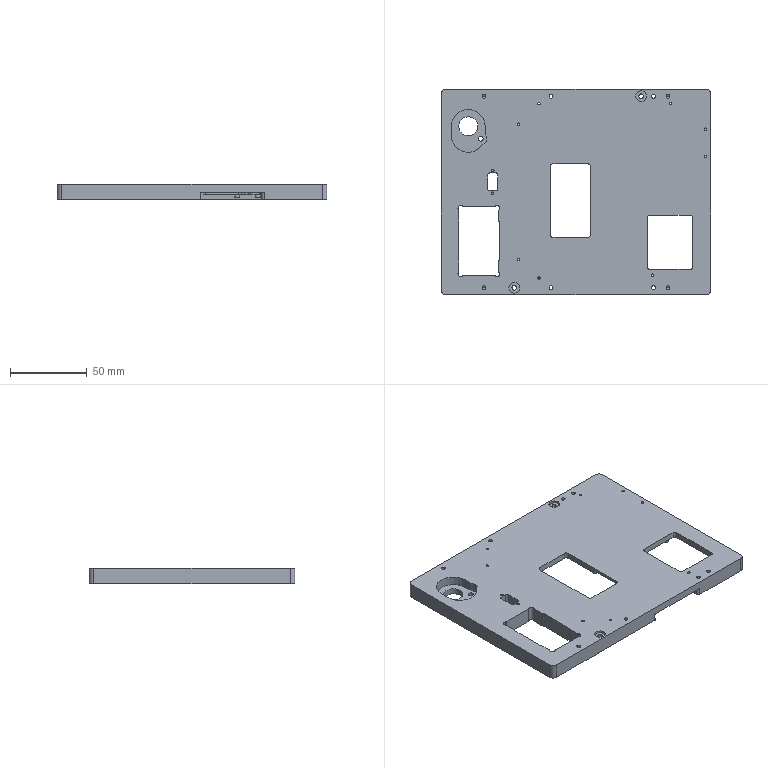NC program | NX | posted with a generic post | part box 176 x 134 x 10 mm
Lines 124 to 1003 of 8914:
(ADAPTIVE_MILLING_COPY , TOOL : D10)
N216 T04 M6
N218 G54
N220 G17 G0 G90 X-60.526 Y-37.7 S9500 M3
N222 G43 Z30. H4
N224 Z1.
N226 G94 G3 X-60.526 Y-37.7 Z0.605 I-2.901 J-3.44 F1000.
N228 X-60.526 Y-37.7 Z0.21 I-2.901 J-3.44
N230 X-60.526 Y-37.7 Z-0.184 I-2.901 J-3.44
N232 X-60.526 Y-37.7 Z-0.579 I-2.901 J-3.44
N234 X-60.526 Y-37.7 Z-0.974 I-2.901 J-3.44
N236 X-60.526 Y-37.7 Z-1.369 I-2.901 J-3.44
N238 X-60.526 Y-37.7 Z-1.764 I-2.901 J-3.44
N240 X-60.526 Y-37.7 Z-2.158 I-2.901 J-3.44
N242 X-60.526 Y-37.7 Z-2.553 I-2.901 J-3.44
N244 X-60.526 Y-37.7 Z-2.948 I-2.901 J-3.44
N246 X-60.526 Y-37.7 Z-3.343 I-2.901 J-3.44
N248 X-60.526 Y-37.7 Z-3.738 I-2.901 J-3.44
N250 X-60.526 Y-37.7 Z-4.133 I-2.901 J-3.44
N252 X-60.526 Y-37.7 Z-4.527 I-2.901 J-3.44
N254 X-60.526 Y-37.7 Z-4.922 I-2.901 J-3.44
N256 X-60.526 Y-37.7 Z-5.317 I-2.901 J-3.44
N258 X-60.526 Y-37.7 Z-5.712 I-2.901 J-3.44
N260 X-60.526 Y-37.7 Z-6.107 I-2.901 J-3.44
N262 X-60.526 Y-37.7 Z-6.501 I-2.901 J-3.44
N264 X-60.526 Y-37.7 Z-6.896 I-2.901 J-3.44
N266 X-60.526 Y-37.7 Z-7.291 I-2.901 J-3.44
N268 X-60.526 Y-37.7 Z-7.686 I-2.901 J-3.44
N270 X-60.526 Y-37.7 Z-8.081 I-2.901 J-3.44
N272 X-60.526 Y-37.7 Z-8.475 I-2.901 J-3.44
N274 X-60.526 Y-37.7 Z-8.87 I-2.901 J-3.44
N276 X-60.526 Y-37.7 Z-9.265 I-2.901 J-3.44
N278 X-60.526 Y-37.7 Z-9.66 I-2.901 J-3.44
N280 X-58.927 Y-41.139 Z-10. R-4.5
N282 X-59.748 Y-43.745 R-4.501 F3500.
N284 X-64.42 Y-36.268 R4.672
N286 X-59.622 Y-44.378 R-4.977
N288 X-65.395 Y-36.044 R5.193
N290 X-59.743 Y-45.214 R-5.474
N292 X-65.843 Y-35.666 R5.72
N294 X-59.62 Y-45.805 R-5.999
N296 X-66.374 Y-35.324 R6.26
N298 X-59.759 Y-46.576 R-6.537
N300 X-66.328 Y-34.682 R6.811
N302 X-59.559 Y-47.121 R-7.099
N304 X-66.7 Y-34.219 R7.384
N306 X-59.276 Y-47.637 R-7.681
N308 X-66.061 Y-33.324 R7.97
N310 X-59.599 Y-48.511 R-8.275
N312 X-57.595 Y-47.115 R8.881
N314 X-55.077 Y-42.632 R7.851
N316 X-55.163 Y-39.012 R27.589
N318 X-63.36 Y-32.265 R8.364
N320 X-71.76 Y-38.033 R8.779
N322 G1 X-71.777 Y-38.154
N324 Y-42.632
N326 G3 X-71.201 Y-45.028 R69.844
N328 X-66.556 Y-49.467 R7.794
N330 X-60.923 Y-49.446 R73.026
N332 X-55.582 Y-45.669 R7.836
N334 X-55.5 Y-45.004 R2.511
N336 G2 X-55.347 Y-43.718 R33.779
N338 G1 X-55.119 Y-42.926
N340 X-55.077 Y-42.632
N342 Y-39.882
N344 G3 X-55.201 Y-37.393 R10.744
N346 X-59.653 Y-32.442 R7.859
N348 X-71.691 Y-36.326 R9.413
N350 G1 X-71.733 Y-36.444
N352 X-71.762 Y-36.566
N354 X-71.777 Y-36.674
N356 Y-38.174
N358 G3 X-71.227 Y-39.126 R1.112
N360 X-70.493 Y-39.275 Z-9.962 R1.332
N362 G1 X-69.254 Y-39.282 Z-9.9
N364 X-57.588 Y-39.349
N366 X-56.035 Y-39.348 Z-9.978
N368 X-55.819 Y-39.293 Z-9.989
N370 X-55.616 Y-39.203 Z-10.
N372 G3 X-55.077 Y-38.257 R1.112
N374 X-55.483 Y-35.569 R5.641
N376 X-61.149 Y-31.221 R8.413
N378 X-71.65 Y-35.064 R9.921
N380 G1 X-71.701 Y-35.178
N382 X-71.74 Y-35.297
N384 X-71.767 Y-35.419
N386 X-71.777 Y-35.493
N388 Y-36.743
N390 G3 X-71.229 Y-37.695 R1.112
N392 X-70.513 Y-37.848 Z-9.963 R1.365
N394 G1 X-69.256 Y-37.882 Z-9.9
N396 X-57.588 Y-38.195
N398 X-56.82 Y-38.218 Z-9.938
N400 X-56.052 Y-38.225 Z-9.977
N402 X-55.827 Y-38.171 Z-9.988
N404 X-55.616 Y-38.078 Z-10.
N406 G3 X-55.077 Y-37.132 R1.112
N408 X-56.62 Y-33.066 R4.979
N410 X-65.601 Y-30.438 R9.835
N412 X-71.544 Y-33.867 R10.035
N414 X-71.777 Y-34.459 R1.804
N416 G1 Y-35.584
N418 G3 X-71.23 Y-36.535 R1.112
N420 X-70.532 Y-36.692 Z-9.964 R1.388
N422 G1 X-69.258 Y-36.751 Z-9.9
N424 X-57.587 Y-37.293
N426 X-56.828 Y-37.332 Z-9.938
N428 X-56.068 Y-37.352 Z-9.976
N430 X-55.835 Y-37.299 Z-9.988
N432 X-55.616 Y-37.204 Z-10.
N434 G3 X-55.077 Y-36.257 R1.112
N436 X-56.507 Y-32.407 R4.688
N438 X-64.492 Y-29.582 R9.928
N440 X-71.39 Y-32.726 R10.586
N442 X-71.777 Y-33.511 R1.491
N444 G1 Y-34.511
N446 G3 X-71.231 Y-35.462 R1.112
N448 X-70.537 Y-35.62 Z-9.964 R1.393
N450 G1 X-69.26 Y-35.686 Z-9.9
N452 X-57.587 Y-36.286
N454 X-56.83 Y-36.329 Z-9.938
N456 X-56.073 Y-36.352 Z-9.976
N458 X-55.838 Y-36.3 Z-9.988
N460 X-55.617 Y-36.204 Z-10.
N462 G3 X-55.077 Y-35.257 R1.112
N464 X-56.412 Y-31.751 R4.409
N466 X-63.51 Y-28.846 R9.893
N468 X-71.115 Y-31.539 R11.237
N470 X-71.777 Y-32.609 R1.829
N472 G1 Y-33.609
N474 G3 X-71.232 Y-34.559 R1.112
N476 X-70.547 Y-34.719 Z-9.964 R1.406
N478 G1 X-69.261 Y-34.798 Z-9.9
N480 X-57.587 Y-35.522
N482 X-56.835 Y-35.573 Z-9.938
N484 X-56.081 Y-35.603 Z-9.975
N486 X-55.842 Y-35.551 Z-9.988
N488 X-55.617 Y-35.454 Z-10.
N490 G3 X-55.077 Y-34.507 R1.112
N492 X-56.413 Y-31.006 R4.337
N494 X-63.408 Y-28.14 R10.025
N496 X-70.99 Y-30.562 R11.468
N498 X-71.777 Y-31.742 R1.951
N500 G1 Y-32.617
N502 G3 X-71.231 Y-33.567 R1.112
N504 X-70.482 Y-33.736 Z-9.961 R1.631
N506 G1 X-69.263 Y-33.832 Z-9.9
N508 X-57.587 Y-34.75
N510 X-56.842 Y-34.813 Z-9.937
N512 X-56.095 Y-34.854 Z-9.975
N514 X-55.849 Y-34.803 Z-9.987
N516 X-55.618 Y-34.705 Z-10.
N518 G3 X-55.077 Y-33.757 R1.112
N520 X-56.421 Y-30.263 R4.261
N522 X-63.059 Y-27.444 R10.076
N524 X-70.846 Y-29.609 R11.73
N526 X-71.755 Y-30.768 R2.336
N528 G1 X-71.777 Y-30.901
N530 Y-31.776
N532 G3 X-71.232 Y-32.726 R1.112
N534 X-70.488 Y-32.896 Z-9.961 R1.643
N536 G1 X-69.264 Y-33. Z-9.9
N538 X-57.586 Y-33.991
N540 X-56.844 Y-34.059 Z-9.937
N542 X-56.101 Y-34.105 Z-9.975
N544 X-55.852 Y-34.054 Z-9.987
N546 X-55.619 Y-33.955 Z-10.
N548 G3 X-55.077 Y-33.007 R1.112
N550 X-56.435 Y-29.521 R4.229
N552 X-62.964 Y-26.734 R10.188
N554 X-70.695 Y-28.674 R11.94
N556 X-71.742 Y-29.881 R2.605
N558 X-71.777 Y-30.943 R12.814
N560 X-71.233 Y-31.892 R1.112
N562 X-70.493 Y-32.064 Z-9.962 R1.655
N564 G1 X-69.265 Y-32.175 Z-9.9
N566 X-57.586 Y-33.234
N568 X-56.847 Y-33.306 Z-9.937
N570 X-56.105 Y-33.355 Z-9.974
N572 X-55.854 Y-33.305 Z-9.987
N574 X-55.619 Y-33.205 Z-10.
N576 G3 X-55.077 Y-32.257 R1.112
N578 X-56.367 Y-28.87 R4.151
N580 X-62.62 Y-26.045 R10.135
N582 X-70.534 Y-27.751 R12.233
N584 X-71.724 Y-28.998 R2.96
N586 X-71.777 Y-30.122 R5.056
N588 X-71.233 Y-31.071 R1.112
N590 X-70.498 Y-31.244 Z-9.962 R1.665
N592 G1 X-69.267 Y-31.362 Z-9.9
N594 X-57.586 Y-32.478
N596 X-56.849 Y-32.553 Z-9.937
N598 X-56.11 Y-32.605 Z-9.974
N600 X-55.857 Y-32.556 Z-9.987
N602 X-55.619 Y-32.455 Z-10.
N604 G3 X-55.077 Y-31.507 R1.112
N606 X-56.389 Y-28.13 R4.127
N608 X-62.652 Y-25.318 R10.251
N610 X-70.47 Y-26.912 R12.253
N612 X-71.699 Y-28.127 R3.313
N614 X-71.777 Y-29.323 R3.839
N616 X-71.234 Y-30.271 R1.112
N618 X-70.501 Y-30.446 Z-9.962 R1.67
N620 G1 X-69.268 Y-30.568 Z-9.9
N622 X-57.586 Y-31.723
N624 X-56.85 Y-31.801 Z-9.937
N626 X-56.112 Y-31.855 Z-9.974
N628 X-55.858 Y-31.806 Z-9.987
N630 X-55.62 Y-31.706 Z-10.
N632 G3 X-55.077 Y-30.757 R1.112
N634 X-56.328 Y-27.482 R4.053
N636 X-62.312 Y-24.634 R10.179
N638 X-70.296 Y-26.011 R12.507
N640 X-71.716 Y-27.375 R3.296
N642 X-71.777 Y-28.523 R4.403
N644 X-71.235 Y-29.471 R1.112
N646 X-70.504 Y-29.646 Z-9.962 R1.677
N648 G1 X-69.27 Y-29.772 Z-9.9
N650 X-57.586 Y-30.969
N652 X-56.852 Y-31.049 Z-9.937
N654 X-56.115 Y-31.105 Z-9.974
N656 X-55.86 Y-31.057 Z-9.987
N658 X-55.62 Y-30.956 Z-10.
N660 G3 X-55.077 Y-30.007 R1.112
N662 X-56.351 Y-26.742 R4.055
N664 X-62.342 Y-23.901 R10.294
N666 X-70.329 Y-25.253 R12.429
N668 X-71.687 Y-26.512 R3.536
N670 X-71.777 Y-27.747 R3.599
N672 X-71.236 Y-28.695 R1.112
N674 X-70.506 Y-28.871 Z-9.962 R1.678
N676 G1 X-69.271 Y-29. Z-9.9
N678 X-57.586 Y-30.216
N680 X-56.853 Y-30.298 Z-9.937
N682 X-56.117 Y-30.356 Z-9.974
N684 X-55.861 Y-30.307 Z-9.987
N686 X-55.62 Y-30.206 Z-10.
N688 G3 X-55.077 Y-29.257 R1.112
N690 X-56.373 Y-26.001 R4.046
N692 X-62.493 Y-23.147 R10.496
N694 X-70.252 Y-24.428 R12.459
N696 X-71.701 Y-25.765 R3.436
N698 X-71.777 Y-26.956 R3.873
N700 X-71.235 Y-27.904 R1.112
N702 X-70.516 Y-28.082 Z-9.963 R1.709
N704 G1 X-69.273 Y-28.226 Z-9.9
N706 X-57.586 Y-29.577
N708 X-56.857 Y-29.667 Z-9.937
N710 X-56.126 Y-29.731 Z-9.973
N712 X-55.866 Y-29.684 Z-9.987
N714 X-55.621 Y-29.582 Z-10.
N716 G3 X-55.077 Y-28.632 R1.112
N718 X-56.397 Y-25.26 R4.101
N720 X-62.521 Y-22.409 R10.57
N722 X-70.282 Y-23.67 R12.37
N724 X-71.714 Y-25.02 R3.246
N726 X-71.777 Y-26.172 R4.315
N728 X-71.236 Y-27.119 R1.112
N730 X-70.519 Y-27.298 Z-9.963 R1.713
N732 G1 X-69.274 Y-27.445 Z-9.9
N734 X-57.586 Y-28.824
N736 X-56.858 Y-28.915 Z-9.937
N738 X-56.128 Y-28.981 Z-9.973
N740 X-55.867 Y-28.934 Z-9.987
N742 X-55.622 Y-28.832 Z-10.
N744 G3 X-55.077 Y-27.882 R1.112
N746 X-56.335 Y-24.61 R4.061
N748 X-62.301 Y-21.707 R10.495
N750 X-70.201 Y-22.851 R12.49
N752 X-71.681 Y-24.159 R3.707
N754 X-71.777 Y-25.397 R3.425
N756 X-71.237 Y-26.344 R1.112
N758 X-70.52 Y-26.524 Z-9.963 R1.714
N760 G1 X-69.276 Y-26.673 Z-9.9
N762 X-57.586 Y-28.071
N764 X-56.859 Y-28.164 Z-9.937
N766 X-56.13 Y-28.231 Z-9.973
N768 X-55.868 Y-28.184 Z-9.987
N770 X-55.622 Y-28.082 Z-10.
N772 G3 X-55.077 Y-27.132 R1.112
N774 X-56.271 Y-23.96 R3.998
N776 X-62.078 Y-21.009 R10.386
N778 X-70.117 Y-22.036 R12.588
N780 X-71.693 Y-23.414 R3.623
N782 X-71.777 Y-24.63 R3.721
N784 X-71.238 Y-25.576 R1.112
N786 X-70.522 Y-25.756 Z-9.963 R1.714
N788 G1 X-69.277 Y-25.907 Z-9.9
N790 X-57.586 Y-27.32
N792 X-56.86 Y-27.413 Z-9.937
N794 X-56.131 Y-27.481 Z-9.973
N796 X-55.868 Y-27.434 Z-9.987
N798 X-55.622 Y-27.332 Z-10.
N800 G3 X-55.077 Y-26.382 R1.112
N802 X-56.377 Y-23.124 R4.098
N804 X-62.471 Y-20.202 R10.732
N806 X-70.139 Y-21.285 R12.45
N808 X-71.703 Y-22.674 R3.454
N810 X-71.777 Y-23.859 R3.92
N812 X-71.238 Y-24.805 R1.112
N814 X-70.531 Y-24.987 Z-9.963 R1.744
N816 G1 X-69.278 Y-25.151 Z-9.9
N818 X-57.586 Y-26.682
N820 X-56.864 Y-26.783 Z-9.936
N822 X-56.139 Y-26.857 Z-9.973
N824 X-55.873 Y-26.811 Z-9.986
N826 X-55.623 Y-26.708 Z-10.
N828 G3 X-55.077 Y-25.757 R1.112
N830 X-56.396 Y-22.382 R4.152
N832 X-62.367 Y-19.48 R10.737
N834 X-70.16 Y-20.532 R12.405
N836 X-71.663 Y-21.816 R3.969
N838 X-71.777 Y-23.092 R3.128
N840 X-71.239 Y-24.037 R1.112
N842 X-70.532 Y-24.22 Z-9.963 R1.744
N844 G1 X-69.28 Y-24.386 Z-9.9
N846 X-57.586 Y-25.931
N848 X-56.865 Y-26.032 Z-9.936
N850 X-56.14 Y-26.107 Z-9.973
N852 X-55.874 Y-26.061 Z-9.986
N854 X-55.623 Y-25.958 Z-10.
N856 G3 X-55.077 Y-25.007 R1.112
N858 X-56.328 Y-21.729 R4.106
N860 X-62.264 Y-18.757 R10.652
N862 X-70.069 Y-19.721 R12.454
N864 X-71.673 Y-21.072 R3.897
N866 X-71.777 Y-22.326 R3.279
N868 X-71.24 Y-23.271 R1.112
N870 X-70.533 Y-23.455 Z-9.963 R1.744
N872 G1 X-69.281 Y-23.622 Z-9.9
N874 X-57.586 Y-25.179
N876 X-56.865 Y-25.281 Z-9.936
N878 X-56.141 Y-25.357 Z-9.973
N880 G3 X-55.624 Y-25.208 Z-10. R1.225
N882 X-55.077 Y-24.257 R1.112
N884 X-56.343 Y-20.986 R4.1
N886 X-62.279 Y-18.013 R10.701
N888 X-70.084 Y-18.97 R12.44
N890 X-71.431 Y-20.051 R3.216
N892 X-71.777 Y-21.472 R5.253
N894 X-71.24 Y-22.417 R1.112
N896 X-70.54 Y-22.602 Z-9.964 R1.765
N898 G1 X-69.283 Y-22.778 Z-9.9
N900 X-57.585 Y-24.42
N902 X-56.184 Y-24.607 Z-9.971
N904 G3 X-55.625 Y-24.458 Z-10. R1.162
N906 X-55.077 Y-23.507 R1.112
N908 X-56.358 Y-20.241 R4.117
N910 X-62.419 Y-17.245 R10.843
N912 X-70.101 Y-18.22 R12.39
N914 X-71.322 Y-19.253 R2.703
N916 X-71.508 Y-20.261 R8.917
N918 X-71.198 Y-21.372 R1.112
N920 X-70.436 Y-21.683 Z-9.958 R1.299
N922 G1 X-69.29 Y-21.869 Z-9.9
N924 X-57.591 Y-23.767
N926 X-56.205 Y-23.982 Z-9.97
N928 G3 X-55.633 Y-23.838 Z-10. R1.16
N930 X-55.077 Y-22.882 R1.112
N932 X-56.373 Y-19.496 R4.179
N934 X-62.557 Y-16.479 R10.927
N936 X-70.002 Y-17.421 R12.259
N938 X-71.285 Y-18.561 R2.598
N940 X-71.413 Y-19.597 R8.909
N942 X-71.052 Y-20.519 R1.116
N944 X-70.309 Y-20.817 Z-9.959 R1.32
N946 G1 X-69.141 Y-21.018 Z-9.9
N948 X-57.586 Y-23.006
N950 X-56.213 Y-23.232 Z-9.97
N952 G3 X-55.631 Y-23.087 Z-10. R1.157
N954 X-55.077 Y-22.132 R1.112
N956 X-56.455 Y-18.689 R4.303
N958 X-62.539 Y-15.739 R10.921
N960 X-69.87 Y-16.612 R12.19
N962 X-71.266 Y-17.817 R3.034
N964 X-71.352 Y-18.915 R3.24
N966 X-70.907 Y-19.798 R1.116
N968 X-70.214 Y-20.031 Z-9.963 R1.366
N970 G1 X-68.967 Y-20.206 Z-9.9
N972 X-57.585 Y-21.808
N974 X-56.941 Y-21.904 Z-9.933
N976 X-56.294 Y-21.976 Z-9.965
N978 G3 X-55.647 Y-21.751 Z-10. R1.145
N980 X-55.257 Y-20.572 R1.108
N982 X-55.701 Y-19.097 R8.228
N984 X-59.336 Y-15.975 R7.604
N986 X-69.431 Y-15.662 R12.888
N988 X-71.212 Y-16.988 R4.158
N990 X-71.352 Y-18.2 R2.531
N992 X-70.854 Y-19.121 R1.115
N994 X-70.116 Y-19.328 Z-9.961 R1.636
N996 G1 X-68.902 Y-19.489 Z-9.9
N998 X-57.753 Y-20.966
N1000 X-57.115 Y-21.056 Z-9.932
N1002 X-56.474 Y-21.122 Z-9.965
N1004 G3 X-55.818 Y-20.88 Z-10. R1.143
N1006 X-55.411 Y-19.919 R1.115
N1008 X-56.909 Y-16.868 R4.192
N1010 X-61.522 Y-14.489 R10.178
N1012 X-67.52 Y-14.527 R124.061
N1014 X-71.098 Y-16.125 R5.682
N1016 X-71.352 Y-16.745 R1.597
N1018 G1 Y-17.495
N1020 G3 X-70.818 Y-18.439 R1.112
N1022 X-70.114 Y-18.625 Z-9.963 R1.753
N1024 G1 X-68.86 Y-18.799 Z-9.9
N1026 X-57.883 Y-20.327
N1028 X-57.219 Y-20.423 Z-9.934
N1030 X-56.552 Y-20.5 Z-9.967
N1032 G3 X-55.936 Y-20.302 Z-10. R1.149
N1034 X-55.47 Y-19.297 R1.112
N1036 X-56.874 Y-16.21 R4.084
N1038 X-59.464 Y-14.506 R7.234
N1040 G1 X-59.583 Y-14.489
N1042 X-61.583
N1044 G3 X-62.179 Y-16.514 R1.101
N1046 G1 X-57.198 Y-19.725
N1048 G3 X-55.502 Y-18.8 R1.102
N1050 X-56.733 Y-15.648 R3.909
N1052 X-58.212 Y-14.524 R4.082
N1054 X-59.646 Y-14.489 R15.119
N1056 X-60.338 Y-16.445 R1.101
N1058 G1 X-57.294 Y-18.906
N1060 G3 X-55.502 Y-18.05 R1.101
N1062 X-57.172 Y-14.614 R3.838
N1064 X-58.47 Y-14.489 R3.013
N1066 X-59.241 Y-16.374 R1.101
N1068 G1 X-57.373 Y-18.21
N1070 G3 X-55.502 Y-17.425 R1.101
N1072 X-56.467 Y-14.704 R3.258
N1074 X-57.671 Y-14.489 R1.91
N1076 X-58.455 Y-16.361 R1.101
N1078 G1 X-57.864 Y-16.97
N1080 X-57.255 Y-17.56
N1082 G3 X-55.502 Y-16.675 R1.101
N1084 X-55.909 Y-14.89 R2.655
N1086 X-57.049 Y-14.489 R1.297
N1088 X-57.839 Y-16.355 R1.101
N1090 G1 X-57.261 Y-16.931
N1092 G3 X-55.502 Y-16.05 R1.101
N1094 X-55.813 Y-14.801 R1.603
N1096 X-56.69 Y-14.489 R1.201
N1098 G1 X-67.022
N1100 G3 X-69.388 Y-14.596 R10.723
N1102 X-71.241 Y-15.769 R2.864
N1104 X-71.352 Y-16.788 R2.415
N1106 X-69.594 Y-17.669 R1.101
N1108 G1 X-67.989 Y-16.471
N1110 G3 X-68.647 Y-14.489 R1.101
N1112 X-70.491 Y-14.703 R4.226
N1114 X-71.352 Y-16.251 R1.39
N1116 X-69.513 Y-17.066 R1.101
N1118 G1 X-69.081 Y-16.679
N1120 X-68.662 Y-16.276
N1122 G3 X-69.522 Y-14.489 R1.101
N1124 X-70.86 Y-14.685 R2.425
N1126 X-71.352 Y-15.802 R1.202
N1128 X-68.865 Y-15.797 R1.244
N1130 X-70.147 Y-14.489 R1.287
N1132 X-71.332 Y-15.401 R1.079
N1134 X-70.654 Y-16.481 R1.007
N1136 G1 X-70.323 Y-16.533 Z-9.983
N1138 X-69.987 Z-9.966
N1140 G2 X-69.281 Y-16.637 Z-9.93 R1.505
N1142 X-68.849 Y-17.048 Z-9.9 R1.047
N1144 G1 X-68.758 Y-17.286
N1146 X-68.723 Y-17.537
N1148 X-68.815 Y-41.972
N1150 G2 X-69.16 Y-42.724 R1.025
N1152 X-69.997 Y-42.968 Z-9.945 R1.137
N1154 G1 X-70.343 Y-42.962 Z-9.962
N1156 X-70.687 Y-42.999 Z-9.979
N1158 X-70.879 Y-43.068 Z-9.99
N1160 X-71.055 Y-43.172 Z-10.
N1162 G3 X-71.443 Y-44.059 R1.014
N1164 X-70.943 Y-46.487 R6.28
N1166 X-68. Y-49.449 R6.448
N1168 X-66.413 Y-49.489 R10.999
N1170 X-65.691 Y-47.559 R1.101
N1172 G1 X-69.531 Y-44.223
N1174 G3 X-71.352 Y-45.054 R1.101
N1176 X-69.896 Y-48.766 R4.582
N1178 X-68.749 Y-49.489 R2.012
N1180 G1 X-67.749
N1182 G3 X-66.958 Y-47.624 R1.101
N1184 G1 X-69.462 Y-45.038
N1186 G3 X-71.352 Y-45.804 R1.101
N1188 X-70.015 Y-49.279 R4.089
N1190 X-69.439 Y-49.489 R1.92
N1192 G1 X-68.689
N1194 G3 X-67.877 Y-47.647 R1.101
N1196 G1 X-69.44 Y-45.937
N1198 G3 X-71.352 Y-46.679 R1.101
N1200 X-70.752 Y-49.04 R3.386
N1202 X-69.942 Y-49.489 R1.225
N1204 G1 X-69.317
N1206 G3 X-68.529 Y-47.622 R1.101
N1208 G1 X-69.053 Y-47.076
N1210 X-69.594 Y-46.547
N1212 G3 X-71.352 Y-47.429 R1.101
N1214 X-71.084 Y-49.002 R2.696
N1216 X-69.873 Y-49.489 R1.267
N1218 X-69.338 Y-47.428 R1.101
N1220 G1 X-69.877 Y-47.144
N1222 G3 X-71.352 Y-48.179 R1.102
N1224 X-70.165 Y-49.489 R1.125
N1226 G1 X-61.42
N1228 G3 X-58.945 Y-49.267 R7.284
N1230 X-55.611 Y-46.75 R6.722
N1232 G1 X-55.564 Y-46.634
N1234 X-55.529 Y-46.514
N1236 X-55.506 Y-46.391
N1238 X-55.502 Y-46.362
N1240 Y-45.237
N1242 G3 X-57.33 Y-44.412 R1.101
N1244 G1 X-60.899 Y-47.565
N1246 G3 X-60.17 Y-49.489 R1.101
N1248 X-57.6 Y-49.123 R5.559
N1250 X-55.641 Y-47.618 R4.794
N1252 X-55.502 Y-46.285 R2.893
N1254 X-57.32 Y-45.452 R1.101
N1256 G1 X-59.763 Y-47.556
N1258 G3 X-59.045 Y-49.489 R1.101
N1260 X-55.998 Y-48.639 R4.266
N1262 X-55.502 Y-47.782 R1.3
N1264 G1 Y-47.157
N1266 G3 X-57.282 Y-46.292 R1.101
N1268 G1 X-58.85 Y-47.525
N1270 G3 X-58.17 Y-49.489 R1.101
N1272 X-56.221 Y-49.19 R3.765
N1274 X-55.502 Y-47.711 R1.383
N1276 X-57.372 Y-46.925 R1.101
N1278 G1 X-57.782 Y-47.322
N1280 X-58.179 Y-47.734
N1282 G3 X-57.295 Y-49.489 R1.101
N1284 X-55.965 Y-49.266 R2.247
N1286 X-55.502 Y-48.177 R1.204
N1288 X-57.898 Y-47.88 R1.217
N1290 X-56.67 Y-49.489 R1.276
N1292 X-55.506 Y-48.454 R1.078
N1294 X-57.238 Y-47.454 R1.42
N1296 G1 Z-7.
N1298 G0 Z30.
N1300 X-99.709 Y-0.062
N1302 Z-9.
N1304 G1 Z-10. F1000.
N1306 X-98.929 Y-0.342 F3500.
N1308 X-98.14 Y-0.598
N1310 G3 X-97.062 Y-0.062 R1.017
N1312 X-96.301 Y3.001 R8.28
N1314 X-96.019 Y12.869 R111.643
N1316 G1 X-96.014 Y15.119
N1318 X-96.011 Y18.994
N1320 X-96.01 Y32.619
N1322 Y67.869
N1324 Y67.994
N1326 X-96.008 Y68.119
N1328 G2 X-93.514 Y72.4 R5.714
N1330 X-88.075 Y74.465 R12.318
N1332 X-79.847 Y74.954 R58.201
N1334 G1 X-78.722 Y74.965
N1336 X-77.347 Y74.974
N1338 X-75.722 Y74.98
N1340 X-73.347 Y74.985
N1342 X-69.222 Y74.987
N1344 X-49.097 Y74.988
N1346 X-16.722
N1348 X-15.097 Y74.995
N1350 X-13.722 Y74.994
N1352 X-12.722 Y74.997
N1354 X-11.222 Y74.995
N1356 X-10.347 Y74.998
N1358 X-9.347 Y74.997
N1360 X-8.097 Y75.
N1362 X-7.097 Y74.998
N1364 X-6.347 Y74.999
N1366 X-5.222 Y74.998
N1368 X-4.597 Y74.997
N1370 X-3.722 Y74.999
N1372 X-2.472 Y74.997
N1374 X-1.597 Y74.999
N1376 X-0.472 Y74.997
N1378 X0.778 Y75.
N1380 X1.528 Y74.999
N1382 X2.403 Y75.
N1384 X2.903 Y75.001
N1386 X4.028 Y74.998
N1388 X5.403 Y75.001
N1390 X6.528 Y74.998
N1392 X7.278 Y75.
N1394 X8.278 Y74.998
N1396 X8.653
N1398 X10.028 Y75.001
N1400 X10.778 Y74.999
N1402 X11.778 Y75.
N1404 X12.403 Y75.001
N1406 X13.528 Y74.998
N1408 X14.528 Y75.001
N1410 X15.903 Y74.997
N1412 X17.153 Y75.
N1414 X18.403 Y74.997
N1416 X19.653 Y75.001
N1418 X20.278 Y74.999
N1420 X21.778 Y75.
N1422 X22.778 Y75.002
N1424 X23.528 Y75.
N1426 X24.528 Y75.001
N1428 X24.903
N1430 X26.153 Y74.998
N1432 X27.028 Y75.
N1434 X28.278 Y74.998
N1436 X29.653 Y75.001
N1438 X30.903 Y74.998
N1440 X32.153 Y75.001
N1442 X33.403 Y74.998
N1444 X34.653 Y75.001
N1446 X35.903 Y74.998
N1448 X36.528 Y74.999
N1450 X38.028 Y74.998
N1452 X39.028 Y74.996
N1454 X39.778 Y74.998
N1456 X40.778 Y74.997
N1458 X41.528 Y74.998
N1460 X42.028 Y74.999
N1462 X43.278 Y74.997
N1464 X44.153 Y74.999
N1466 X44.778 Y74.998
N1468 X45.528 Y74.997
N1470 X46.528 Y74.999
N1472 X47.278 Y74.998
N1474 X48.403 Y75.
N1476 X48.903 Y75.001
N1478 X50.153 Y74.998
N1480 X50.903 Y74.999
N1482 X51.903 Y74.998
N1484 X52.403 Y74.997
N1486 X53.278 Y74.999
N1488 X54.278 Y74.998
N1490 X55.278 Y75.
N1492 X56.403 Y74.998
N1494 X57.653 Y75.
N1496 X58.278 Y74.999
N1498 X59.778 Y75.
N1500 X60.403 Y75.001
N1502 X61.403 Y74.999
N1504 X62.153 Y75.
N1506 X63.278 Y74.999
N1508 X63.653 Y74.998
N1510 X64.653 Y75.
N1512 X65.403 Y74.999
N1514 X66.528 Y75.
N1516 X67.153
N1518 X68.153 Y74.997
N1520 X68.778 Y74.999
N1522 X70.278 Y74.998
N1524 X70.903 Y74.997
N1526 X72.028 Y74.999
N1528 X73.028 Y74.997
N1530 X74.278 Y75.
N1532 X75.153 Y74.998
N1534 X76.403 Y75.
N1536 X77.153 Y74.999
N1538 X78.278 Y75.001
N1540 X78.903 Y75.
N1542 X79.903 Y74.998
N1544 X80.653 Y74.999
N1546 X81.653 Y74.998
N1548 X82.278 Y74.997
N1550 X83.528 Y75.
N1552 X84.403 Y74.998
N1554 X85.403 Y75.
N1556 X85.778 Y75.001
N1558 X86.903 Y74.998
N1560 G2 X89.897 Y74.905 R17.614
N1562 X93.968 Y71.64 R6.427
N1564 X95.666 Y65.543 R15.399
N1566 X95.976 Y55.927 R109.112
N1568 G1 X95.982 Y54.052
N1570 X95.986 Y51.177
N1572 X95.988 Y45.427
N1574 X95.989 Y-6.448
N1576 X95.995 Y-7.948
N1578 X95.994 Y-9.448
N1580 X95.996 Y-10.073
N1582 Y-11.198
N1584 X95.995 Y-11.823
N1586 X95.998 Y-12.698
N1588 X95.997 Y-13.698
N1590 X95.999 Y-14.698
N1592 X95.997 Y-15.948
N1594 X95.999 Y-16.573
N1596 X95.998 Y-17.948
N1598 X95.997 Y-18.448
N1600 X95.999 Y-19.448
N1602 X95.997 Y-20.573
N1604 X95.999 Y-21.323
N1606 X95.998 Y-22.198
N1608 X95.997 Y-22.698
N1610 X95.999 Y-23.573
N1612 X95.997 Y-24.948
N1614 X95.999 Y-25.698
N1616 X95.998 Y-26.573
N1618 Y-26.948
N1620 X96. Y-28.073
N1622 X95.998 Y-29.073
N1624 X96.001 Y-30.323
N1626 X96. Y-30.948
N1628 X96.001 Y-32.448
N1630 X96.002 Y-33.073
N1632 X96. Y-33.948
N1634 X96.001 Y-35.073
N1636 X96. Y-35.823
N1638 X96.001 Y-37.073
N1640 X95.998 Y-38.323
N1642 X95.999 Y-38.948
N1644 X95.998 Y-40.323
N1646 X95.997 Y-40.948
N1648 X95.999 Y-41.573
N1650 X95.998 Y-42.948
N1652 X95.997 Y-43.448
N1654 X96. Y-44.448
N1656 X95.997 Y-45.573
N1658 X95.999 Y-46.323
N1660 X95.998 Y-47.198
N1662 Y-47.698
N1664 X95.999 Y-48.573
N1666 X95.997 Y-49.948
N1668 X95.999 Y-50.698
N1670 X95.998 Y-51.573
N1672 Y-51.948
N1674 X96. Y-53.073
N1676 X95.998 Y-54.073
N1678 X96.001 Y-55.198
N1680 X95.999 Y-55.948
N1682 X96. Y-56.823
N1684 X96.001 Y-57.198
N1686 X95.998 Y-58.573
N1688 X96.001 Y-59.823
N1690 X95.998 Y-60.948
N1692 X95.999 Y-61.573
N1694 X95.998 Y-62.948
N1696 X95.997 Y-63.573
N1698 X96. Y-64.573
N1700 X95.997 Y-65.823
N1702 X96. Y-67.073
N1704 X95.997 Y-68.073
N1706 X95.995 Y-68.198
N1708 X95.987 Y-68.323
N1710 X95.975 Y-68.447
N1712 G2 X93.13 Y-72.662 R6.037
N1714 X87.489 Y-74.552 R13.48
N1716 X78.879 Y-74.964 R71.866
N1718 G1 X77.629 Y-74.972
N1720 X76.004 Y-74.979
N1722 X73.754 Y-74.984
N1724 X70.004 Y-74.987
N1726 X57.754 Y-74.988
N1728 X-88.996
N1730 G2 X-93.326 Y-72.588 R5.655
N1732 X-95.445 Y-67.172 R12.051
N1734 X-95.955 Y-58.82 R57.462
N1736 G1 X-95.965 Y-57.82
N1738 X-95.973 Y-56.57
N1740 X-95.98 Y-54.945
N1742 X-95.985 Y-52.57
N1744 X-95.988 Y-48.695
N1746 X-95.989 Y-35.32
N1748 Y-3.82
N1750 X-95.988 Y-3.695
N1752 X-95.985 Y-3.57
N1754 X-95.979 Y-3.32
N1756 X-95.974 Y-3.195
N1758 G2 X-95.342 Y3.021 R351.311
N1760 G3 X-95.029 Y16.265 R190.267
N1762 G1 X-95.024 Y19.14
N1764 X-95.022 Y24.265
N1766 X-95.021 Y64.89
N1768 X-95.019 Y65.015
N1770 X-95.017 Y65.14
N1772 X-95.005 Y65.389
N1774 G2 X-91.224 Y71.394 R7.721
N1776 X-84.736 Y73.499 R15.865
N1778 X-75.627 Y73.946 R79.266
N1780 G1 X-74.502 Y73.956
N1782 X-73.002 Y73.964
N1784 X-71.002 Y73.97
N1786 X-68.127 Y73.975
N1788 X-62.752 Y73.977
N1790 X-19.752 Y73.978
N1792 X-18.127 Y73.987
N1794 X-16.502
N1796 X-15.502 Y73.991
N1798 X-14.877
N1800 X-14.127 Y73.99
N1802 X-13.127 Y73.994
N1804 X-12.502
N1806 X-11.877 Y73.993
N1808 X-10.877 Y73.996
N1810 X-9.752 Y73.995
N1812 X-8.627 Y73.998
N1814 X-7.502 Y73.996
N1816 X-6.252 Y73.999
N1818 X-5.502 Y73.997
N1820 X-4.252 Y73.998
N1822 X-3.752 Y73.999
N1824 X-3.002 Y73.998
N1826 X-1.877 Y73.999
N1828 X-1.252
N1830 X-0.502 Y73.998
N1832 X0.498 Y74.
N1834 X1.373 Y73.998
N1836 X2.623 Y74.
N1838 X3.623 Y73.998
N1840 X4.873 Y74.001
N1842 X6.123 Y73.998
N1844 X7.123 Y74.
N1846 X8.248 Y73.998
N1848 X9.623 Y74.001
N1850 X10.623 Y73.999
N1852 X11.873 Y74.001
N1854 X13.248 Y73.998
N1856 X14.248 Y74.
N1858 X15.248 Y73.998
N1860 X15.623 Y73.997
N1862 X16.873 Y74.
N1864 X17.623 Y73.999
N1866 X18.873 Y74.
N1868 X19.873 Y74.003
N1870 X21.123 Y74.
N1872 X22.248 Y74.002
N1874 X23.373 Y73.999
N1876 X24.748 Y74.002
N1878 X25.623 Y73.999
N1880 X26.623 Y74.001
N1882 X27.248
N1884 X27.873 Y73.999
N1886 X28.998 Y74.001
N1888 X29.623
N1890 X30.623 Y73.998
N1892 X31.873 Y74.001
N1894 X33.123 Y73.998
N1896 X33.873 Y73.999
N1898 X35.123 Y73.998
N1900 X35.998 Y73.995
N1902 X37.373 Y73.999
N1904 X38.123 Y73.997
N1906 X39.248 Y73.999
N1908 X39.623
N1910 X40.748 Y73.997
N1912 X41.873 Y73.999
N1914 X42.748 Y73.997
N1916 X43.998 Y73.999
N1918 X44.873 Y73.997
N1920 X46.123 Y74.
N1922 X47.498 Y73.997
N1924 X48.623 Y74.
N1926 X49.498 Y73.998
N1928 X50.373 Y73.999
N1930 X50.748
N1932 X51.748 Y73.998
N1934 X52.873 Y74.
N1936 X53.623 Y73.998
N1938 X54.873 Y73.999
N1940 X55.373 Y74.
N1942 X56.248 Y73.999
N1944 X56.998 Y74.
N1946 X57.498 Y74.001
N1948 X58.623 Y73.999
N1950 X59.873 Y74.001
N1952 X60.748 Y73.999
N1954 X61.623 Y74.
N1956 X62.123 Y74.001
N1958 X63.373 Y73.998
N1960 X64.248 Y74.
N1962 X65.373 Y73.998
N1964 X66.623 Y74.
N1966 X67.748 Y73.997
N1968 X68.998 Y74.